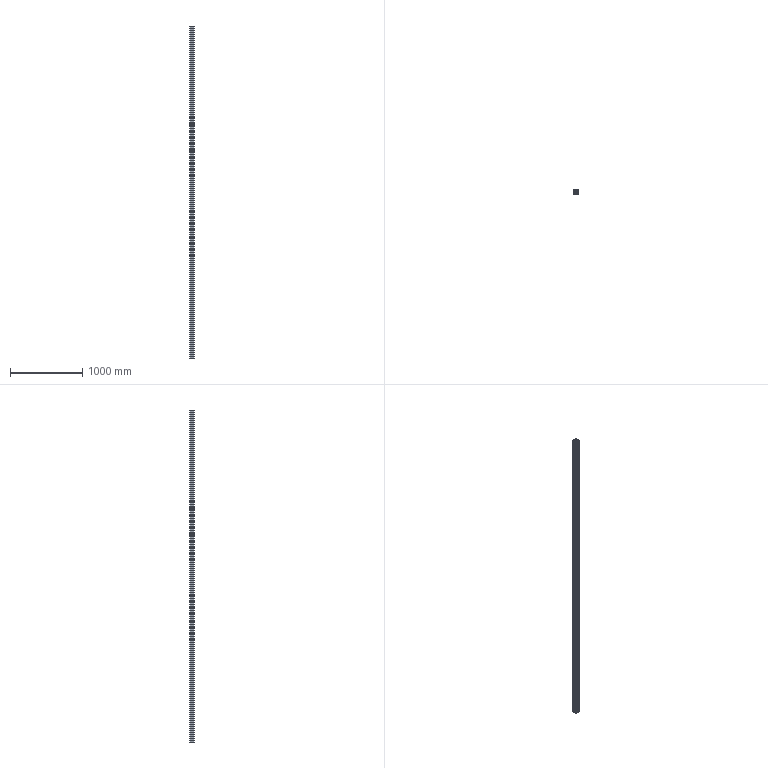Part | NX | features BREP 1 | 1 solid | 162 faces | box 60 x 60 x 4600 mm | volume 7035763 mm3 | plane 130 | cylinder 32 | commonest cylinder face diameters 2 x16 6.8 x8 4 x4 6 x4